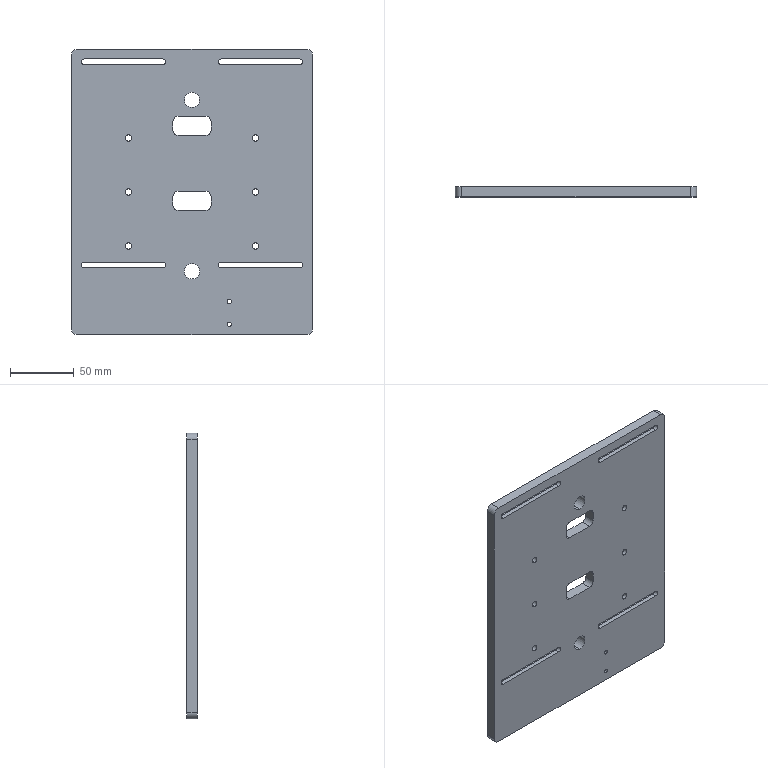Part | STEP file | 0-19-08 Connecting plate | 1 solid | 82 faces | box 190 x 8 x 225 mm | volume 317897 mm3 | cylinder 48 | plane 34 | commonest cylinder face diameters 8 x16 5 x12 4.5 x8 3.3 x4 10 x4 12 x4